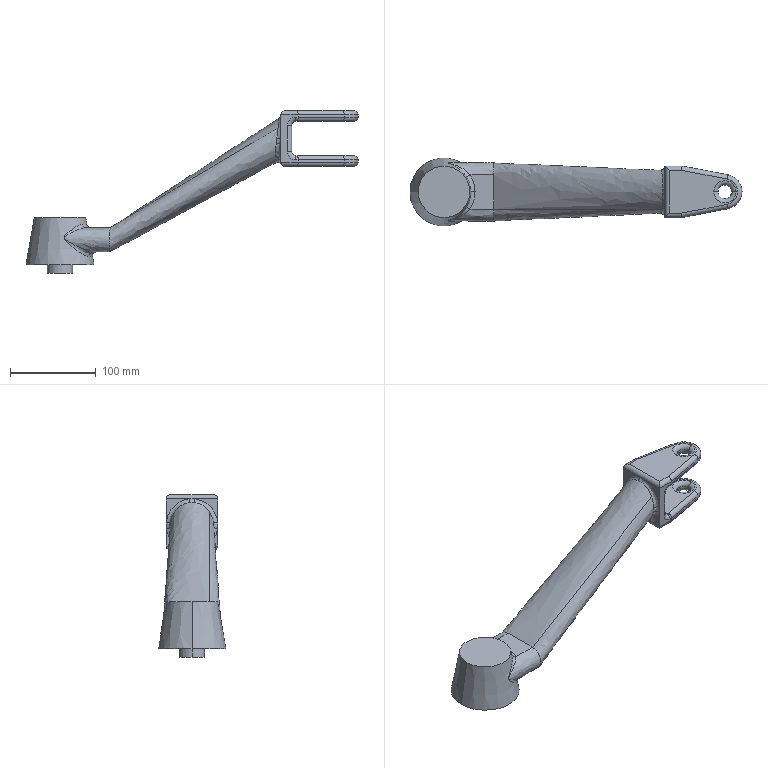Part | SolidWorks | 1 solid | 87 faces | box 387.698 x 79.396 x 190 mm | volume 762316 mm3 | cylinder 30 | torus 21 | plane 20 | spline 14 | cone 2 | commonest cylinder face diameters 10 x22 16 x4 30 x2 40 x2